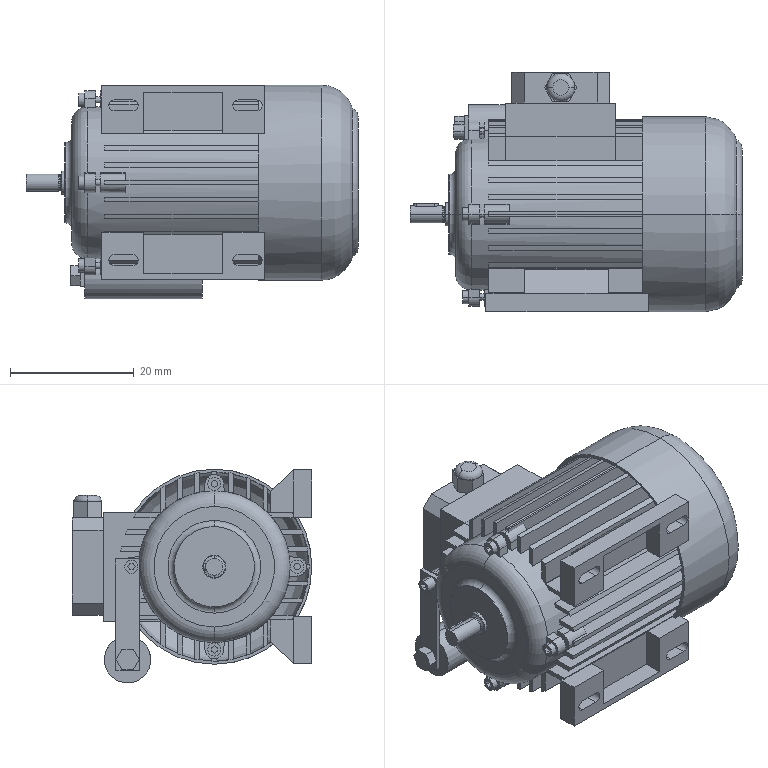Part | SolidWorks | features ICE 20, Fillet 3, CirPattern 2, Revolution 2, LPattern 1, Scale 1 | 6 solids | 596 faces | box 53.612 x 38.693 x 34.5 mm | volume 25264 mm3 | plane 469 | cylinder 105 | torus 20 | cone 2 | commonest cylinder face diameters 24.5 x19 30.5 x12 30.501 x12 3 x10 30.619 x10 1 x8